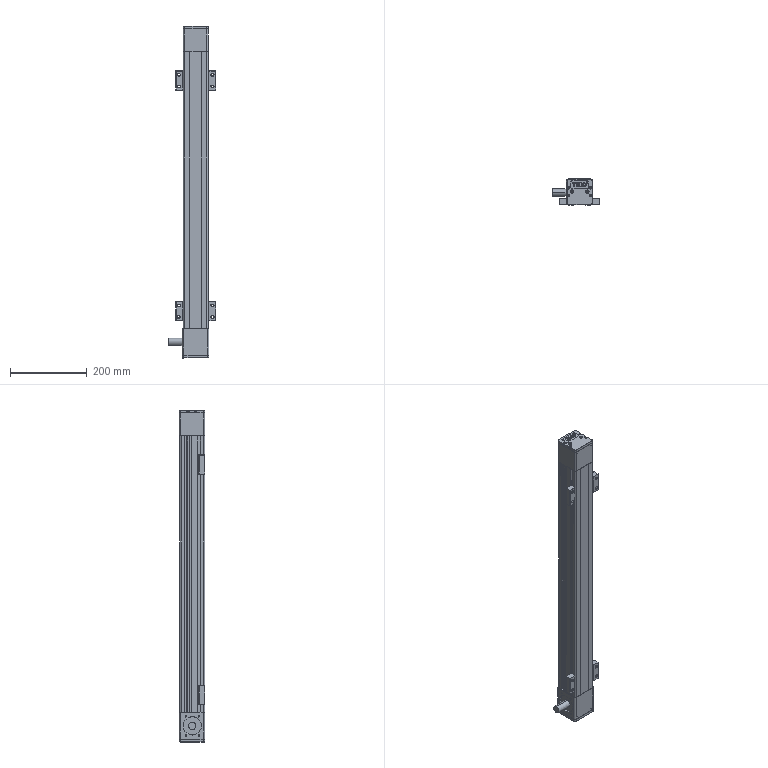Part | SolidWorks | 10 solids | 1258 faces | box 123 x 66.8 x 864 mm | volume 3505638 mm3 | plane 673 | cylinder 322 | cone 230 | spline 33 | commonest cylinder face diameters 0.6 x48 6 x36 5.5 x32 3.3 x24 8 x24 10 x18